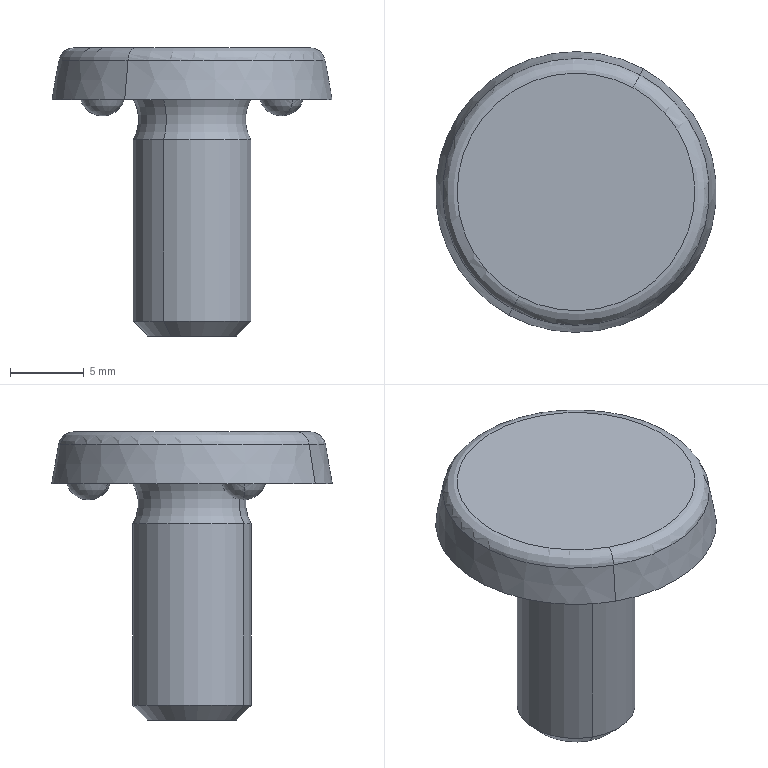Part | 1 solid | 19 faces | box 19 x 19 x 19.5 mm | volume 1712 mm3 | sphere 6 | cone 4 | torus 4 | plane 3 | cylinder 2 | commonest cylinder face diameters 8 x2